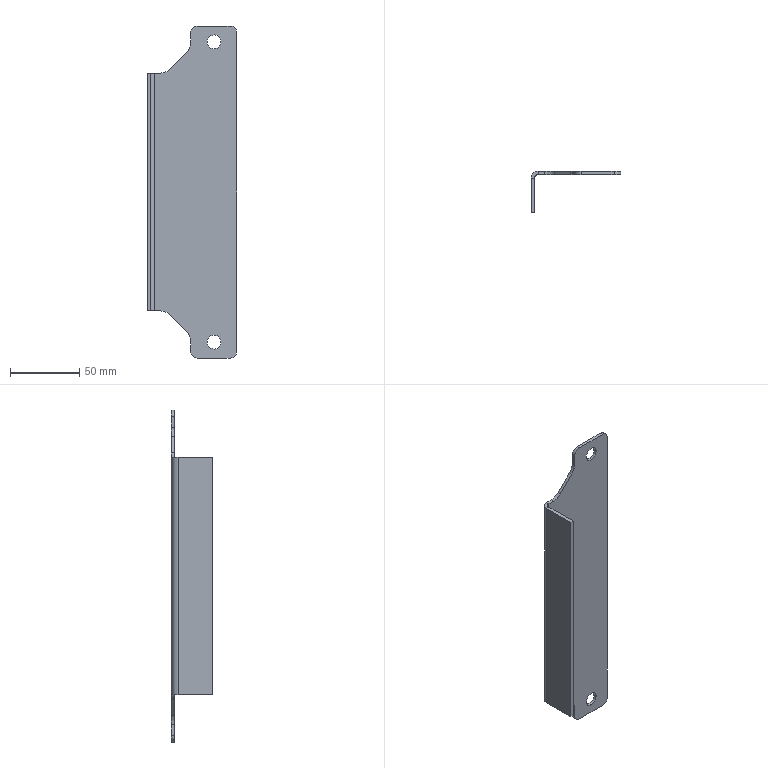Part | SolidWorks | features BaseBody 1, FlatPattern 1, SheetMetal 1, SolidToSheetMetal 1 | 1 solid | 32 faces | box 65 x 30 x 240 mm | volume 41523 mm3 | plane 18 | cylinder 14 | commonest cylinder face diameters 10 x8 20 x4 6 x1 10.6 x1
STEP:
#1=CARTESIAN_POINT('',(1146.2,76.5,704.5));
#2=VERTEX_POINT('',#1);
#3=CARTESIAN_POINT('',(1146.2,76.5,694.5));
#4=VERTEX_POINT('',#3);
#5=CARTESIAN_POINT('',(1146.2,76.5,699.5));
#6=DIRECTION('',(0.,-1.,0.));
#7=DIRECTION('',(0.,0.,-1.));
#8=AXIS2_PLACEMENT_3D('',#5,#6,#7);
#9=CIRCLE('',#8,5.);
#10=EDGE_CURVE('',#2,#4,#9,.T.);
#11=ORIENTED_EDGE('',*,*,#10,.T.);
#12=CARTESIAN_POINT('',(1146.2,78.8,694.5));
#13=VERTEX_POINT('',#12);
#14=CARTESIAN_POINT('',(1146.2,76.5,694.5));
#15=DIRECTION('',(0.,1.,0.));
#16=VECTOR('',#15,1000.);
#17=LINE('',#14,#16);
#18=EDGE_CURVE('',#4,#13,#17,.T.);
#19=ORIENTED_EDGE('',*,*,#18,.T.);
#20=CARTESIAN_POINT('',(1146.2,78.8,704.5));
#21=VERTEX_POINT('',#20);
#22=CARTESIAN_POINT('',(1146.2,78.8,699.5));
#23=DIRECTION('',(0.,-1.,0.));
#24=DIRECTION('',(0.,0.,-1.));
#25=AXIS2_PLACEMENT_3D('',#22,#23,#24);
#26=CIRCLE('',#25,5.);
#27=EDGE_CURVE('',#21,#13,#26,.T.);
#28=ORIENTED_EDGE('',*,*,#27,.F.);
#29=CARTESIAN_POINT('',(1146.2,76.5,704.5));
#30=DIRECTION('',(0.,1.,0.));
#31=VECTOR('',#30,1000.);
#32=LINE('',#29,#31);
#33=EDGE_CURVE('',#2,#21,#32,.T.);
#34=ORIENTED_EDGE('',*,*,#33,.F.);
#35=EDGE_LOOP('',(#11,#19,#28,#34));
#36=FACE_OUTER_BOUND('',#35,.T.);
#37=CARTESIAN_POINT('',(1146.2,76.5,699.5));
#38=DIRECTION('',(0.,1.,0.));
#39=DIRECTION('',(0.,0.,1.));
#40=AXIS2_PLACEMENT_3D('',#37,#38,#39);
#41=CYLINDRICAL_SURFACE('',#40,5.);
#42=ADVANCED_FACE('',(#36),#41,.F.);
#43=CARTESIAN_POINT('',(1146.2,76.5,487.5));
#44=VERTEX_POINT('',#43);
#45=CARTESIAN_POINT('',(1146.2,76.5,477.5));
#46=VERTEX_POINT('',#45);
#47=CARTESIAN_POINT('',(1146.2,76.5,482.5));
#48=DIRECTION('',(0.,-1.,0.));
#49=DIRECTION('',(0.,0.,1.));
#50=AXIS2_PLACEMENT_3D('',#47,#48,#49);
#51=CIRCLE('',#50,5.);
#52=EDGE_CURVE('',#44,#46,#51,.T.);
#53=ORIENTED_EDGE('',*,*,#52,.T.);
#54=CARTESIAN_POINT('',(1146.2,78.8,477.5));
#55=VERTEX_POINT('',#54);
#56=CARTESIAN_POINT('',(1146.2,76.5,477.5));
#57=DIRECTION('',(0.,1.,0.));
#58=VECTOR('',#57,1000.);
#59=LINE('',#56,#58);
#60=EDGE_CURVE('',#46,#55,#59,.T.);
#61=ORIENTED_EDGE('',*,*,#60,.T.);
#62=CARTESIAN_POINT('',(1146.2,78.8,487.5));
#63=VERTEX_POINT('',#62);
#64=CARTESIAN_POINT('',(1146.2,78.8,482.5));
#65=DIRECTION('',(0.,-1.,0.));
#66=DIRECTION('',(0.,0.,1.));
#67=AXIS2_PLACEMENT_3D('',#64,#65,#66);
#68=CIRCLE('',#67,5.);
#69=EDGE_CURVE('',#63,#55,#68,.T.);
#70=ORIENTED_EDGE('',*,*,#69,.F.);
#71=CARTESIAN_POINT('',(1146.2,76.5,487.5));
#72=DIRECTION('',(0.,1.,0.));
#73=VECTOR('',#72,1000.);
#74=LINE('',#71,#73);
#75=EDGE_CURVE('',#44,#63,#74,.T.);
#76=ORIENTED_EDGE('',*,*,#75,.F.);
#77=EDGE_LOOP('',(#53,#61,#70,#76));
#78=FACE_OUTER_BOUND('',#77,.T.);
#79=CARTESIAN_POINT('',(1146.2,76.5,482.5));
#80=DIRECTION('',(0.,1.,0.));
#81=DIRECTION('',(0.,0.,1.));
#82=AXIS2_PLACEMENT_3D('',#79,#80,#81);
#83=CYLINDRICAL_SURFACE('',#82,5.);
#84=ADVANCED_FACE('',(#78),#83,.F.);
#85=CARTESIAN_POINT('',(1107.528,78.8,505.));
#86=VERTEX_POINT('',#85);
#87=CARTESIAN_POINT('',(1107.528,76.5,505.));
#88=VERTEX_POINT('',#87);
#89=CARTESIAN_POINT('',(1107.528,76.5,505.));
#90=DIRECTION('',(0.,-1.,0.));
#91=VECTOR('',#90,1000.);
#92=LINE('',#89,#91);
#93=EDGE_CURVE('',#86,#88,#92,.T.);
#94=ORIENTED_EDGE('',*,*,#93,.F.);
#95=CARTESIAN_POINT('',(1114.599,78.8,502.071));
#96=VERTEX_POINT('',#95);
#97=CARTESIAN_POINT('',(1107.528,78.8,495.));
#98=DIRECTION('',(0.,-1.,0.));
#99=DIRECTION('',(0.,0.,-1.));
#100=AXIS2_PLACEMENT_3D('',#97,#98,#99);
#101=CIRCLE('',#100,10.);
#102=EDGE_CURVE('',#96,#86,#101,.T.);
#103=ORIENTED_EDGE('',*,*,#102,.F.);
#104=CARTESIAN_POINT('',(1114.599,76.5,502.071));
#105=VERTEX_POINT('',#104);
#106=CARTESIAN_POINT('',(1114.599,76.5,502.071));
#107=DIRECTION('',(0.,-1.,0.));
#108=VECTOR('',#107,1000.);
#109=LINE('',#106,#108);
#110=EDGE_CURVE('',#96,#105,#109,.T.);
#111=ORIENTED_EDGE('',*,*,#110,.T.);
#112=CARTESIAN_POINT('',(1107.528,76.5,495.));
#113=DIRECTION('',(0.,-1.,0.));
#114=DIRECTION('',(0.,0.,-1.));
#115=AXIS2_PLACEMENT_3D('',#112,#113,#114);
#116=CIRCLE('',#115,10.);
#117=EDGE_CURVE('',#105,#88,#116,.T.);
#118=ORIENTED_EDGE('',*,*,#117,.T.);
#119=EDGE_LOOP('',(#94,#103,#111,#118));
#120=FACE_OUTER_BOUND('',#119,.T.);
#121=CARTESIAN_POINT('',(1107.528,76.5,495.));
#122=DIRECTION('',(0.,1.,0.));
#123=DIRECTION('',(0.,0.,1.));
#124=AXIS2_PLACEMENT_3D('',#121,#122,#123);
#125=CYLINDRICAL_SURFACE('',#124,10.);
#126=ADVANCED_FACE('',(#120),#125,.F.);
#127=ORIENTED_EDGE('',*,*,#110,.F.);
#128=CARTESIAN_POINT('',(1126.271,78.8,490.399));
#129=VERTEX_POINT('',#128);
#130=CARTESIAN_POINT('',(1126.271,78.8,490.399));
#131=DIRECTION('',(-0.7071,0.,0.7071));
#132=VECTOR('',#131,1000.);
#133=LINE('',#130,#132);
#134=EDGE_CURVE('',#129,#96,#133,.T.);
#135=ORIENTED_EDGE('',*,*,#134,.F.);
#136=CARTESIAN_POINT('',(1126.271,76.5,490.399));
#137=VERTEX_POINT('',#136);
#138=CARTESIAN_POINT('',(1126.271,76.5,490.399));
#139=DIRECTION('',(0.,-1.,0.));
#140=VECTOR('',#139,1000.);
#141=LINE('',#138,#140);
#142=EDGE_CURVE('',#129,#137,#141,.T.);
#143=ORIENTED_EDGE('',*,*,#142,.T.);
#144=CARTESIAN_POINT('',(1126.271,76.5,490.399));
#145=DIRECTION('',(-0.7071,0.,0.7071));
#146=VECTOR('',#145,1000.);
#147=LINE('',#144,#146);
#148=EDGE_CURVE('',#137,#105,#147,.T.);
#149=ORIENTED_EDGE('',*,*,#148,.T.);
#150=EDGE_LOOP('',(#127,#135,#143,#149));
#151=FACE_OUTER_BOUND('',#150,.T.);
#152=CARTESIAN_POINT('',(1126.271,76.5,490.399));
#153=DIRECTION('',(-0.7071,0.,-0.7071));
#154=DIRECTION('',(-0.7071,0.,0.7071));
#155=AXIS2_PLACEMENT_3D('',#152,#153,#154);
#156=PLANE('',#155);
#157=ADVANCED_FACE('',(#151),#156,.T.);
#158=ORIENTED_EDGE('',*,*,#142,.F.);
#159=CARTESIAN_POINT('',(1129.2,78.8,483.328));
#160=VERTEX_POINT('',#159);
#161=CARTESIAN_POINT('',(1119.2,78.8,483.328));
#162=DIRECTION('',(0.,-1.,0.));
#163=DIRECTION('',(1.,0.,0.));
#164=AXIS2_PLACEMENT_3D('',#161,#162,#163);
#165=CIRCLE('',#164,10.);
#166=EDGE_CURVE('',#160,#129,#165,.T.);
#167=ORIENTED_EDGE('',*,*,#166,.F.);
#168=CARTESIAN_POINT('',(1129.2,76.5,483.328));
#169=VERTEX_POINT('',#168);
#170=CARTESIAN_POINT('',(1129.2,76.5,483.328));
#171=DIRECTION('',(0.,-1.,0.));
#172=VECTOR('',#171,1000.);
#173=LINE('',#170,#172);
#174=EDGE_CURVE('',#160,#169,#173,.T.);
#175=ORIENTED_EDGE('',*,*,#174,.T.);
#176=CARTESIAN_POINT('',(1119.2,76.5,483.328));
#177=DIRECTION('',(0.,-1.,0.));
#178=DIRECTION('',(1.,0.,0.));
#179=AXIS2_PLACEMENT_3D('',#176,#177,#178);
#180=CIRCLE('',#179,10.);
#181=EDGE_CURVE('',#169,#137,#180,.T.);
#182=ORIENTED_EDGE('',*,*,#181,.T.);
#183=EDGE_LOOP('',(#158,#167,#175,#182));
#184=FACE_OUTER_BOUND('',#183,.T.);
#185=CARTESIAN_POINT('',(1119.2,76.5,483.328));
#186=DIRECTION('',(0.,1.,0.));
#187=DIRECTION('',(0.,0.,1.));
#188=AXIS2_PLACEMENT_3D('',#185,#186,#187);
#189=CYLINDRICAL_SURFACE('',#188,10.);
#190=ADVANCED_FACE('',(#184),#189,.F.);
#191=ORIENTED_EDGE('',*,*,#174,.F.);
#192=CARTESIAN_POINT('',(1129.2,78.8,476.));
#193=VERTEX_POINT('',#192);
#194=CARTESIAN_POINT('',(1129.2,78.8,711.));
#195=DIRECTION('',(0.,0.,1.));
#196=VECTOR('',#195,1000.);
#197=LINE('',#194,#196);
#198=EDGE_CURVE('',#193,#160,#197,.T.);
#199=ORIENTED_EDGE('',*,*,#198,.F.);
#200=CARTESIAN_POINT('',(1129.2,76.5,476.));
#201=VERTEX_POINT('',#200);
#202=CARTESIAN_POINT('',(1129.2,76.5,476.));
#203=DIRECTION('',(0.,-1.,0.));
#204=VECTOR('',#203,1000.);
#205=LINE('',#202,#204);
#206=EDGE_CURVE('',#193,#201,#205,.T.);
#207=ORIENTED_EDGE('',*,*,#206,.T.);
#208=CARTESIAN_POINT('',(1129.2,76.5,591.));
#209=DIRECTION('',(0.,0.,1.));
#210=VECTOR('',#209,1000.);
#211=LINE('',#208,#210);
#212=EDGE_CURVE('',#201,#169,#211,.T.);
#213=ORIENTED_EDGE('',*,*,#212,.T.);
#214=EDGE_LOOP('',(#191,#199,#207,#213));
#215=FACE_OUTER_BOUND('',#214,.T.);
#216=CARTESIAN_POINT('',(1129.2,76.5,591.));
#217=DIRECTION('',(-1.,0.,0.));
#218=DIRECTION('',(0.,0.,1.));
#219=AXIS2_PLACEMENT_3D('',#216,#217,#218);
#220=PLANE('',#219);
#221=ADVANCED_FACE('',(#215),#220,.T.);
#222=ORIENTED_EDGE('',*,*,#206,.F.);
#223=CARTESIAN_POINT('',(1134.2,78.8,471.));
#224=VERTEX_POINT('',#223);
#225=CARTESIAN_POINT('',(1134.2,78.8,476.));
#226=DIRECTION('',(0.,1.,0.));
#227=DIRECTION('',(0.,0.,1.));
#228=AXIS2_PLACEMENT_3D('',#225,#226,#227);
#229=CIRCLE('',#228,5.);
#230=EDGE_CURVE('',#224,#193,#229,.T.);
#231=ORIENTED_EDGE('',*,*,#230,.F.);
#232=CARTESIAN_POINT('',(1134.2,76.5,471.));
#233=VERTEX_POINT('',#232);
#234=CARTESIAN_POINT('',(1134.2,76.5,471.));
#235=DIRECTION('',(0.,-1.,0.));
#236=VECTOR('',#235,1000.);
#237=LINE('',#234,#236);
#238=EDGE_CURVE('',#224,#233,#237,.T.);
#239=ORIENTED_EDGE('',*,*,#238,.T.);
#240=CARTESIAN_POINT('',(1134.2,76.5,476.));
#241=DIRECTION('',(0.,1.,0.));
#242=DIRECTION('',(0.,0.,1.));
#243=AXIS2_PLACEMENT_3D('',#240,#241,#242);
#244=CIRCLE('',#243,5.);
#245=EDGE_CURVE('',#233,#201,#244,.T.);
#246=ORIENTED_EDGE('',*,*,#245,.T.);
#247=EDGE_LOOP('',(#222,#231,#239,#246));
#248=FACE_OUTER_BOUND('',#247,.T.);
#249=CARTESIAN_POINT('',(1134.2,76.5,476.));
#250=DIRECTION('',(0.,1.,0.));
#251=DIRECTION('',(0.,0.,1.));
#252=AXIS2_PLACEMENT_3D('',#249,#250,#251);
#253=CYLINDRICAL_SURFACE('',#252,5.);
#254=ADVANCED_FACE('',(#248),#253,.T.);
#255=ORIENTED_EDGE('',*,*,#238,.F.);
#256=CARTESIAN_POINT('',(1157.7,78.8,471.));
#257=VERTEX_POINT('',#256);
#258=CARTESIAN_POINT('',(1103.,78.8,471.));
#259=DIRECTION('',(-1.,0.,0.));
#260=VECTOR('',#259,1000.);
#261=LINE('',#258,#260);
#262=EDGE_CURVE('',#257,#224,#261,.T.);
#263=ORIENTED_EDGE('',*,*,#262,.F.);
#264=CARTESIAN_POINT('',(1157.7,76.5,471.));
#265=VERTEX_POINT('',#264);
#266=CARTESIAN_POINT('',(1157.7,76.5,471.));
#267=DIRECTION('',(0.,-1.,0.));
#268=VECTOR('',#267,1000.);
#269=LINE('',#266,#268);
#270=EDGE_CURVE('',#257,#265,#269,.T.);
#271=ORIENTED_EDGE('',*,*,#270,.T.);
#272=CARTESIAN_POINT('',(1132.85,76.5,471.));
#273=DIRECTION('',(-1.,0.,0.));
#274=VECTOR('',#273,1000.);
#275=LINE('',#272,#274);
#276=EDGE_CURVE('',#265,#233,#275,.T.);
#277=ORIENTED_EDGE('',*,*,#276,.T.);
#278=EDGE_LOOP('',(#255,#263,#271,#277));
#279=FACE_OUTER_BOUND('',#278,.T.);
#280=CARTESIAN_POINT('',(1132.85,76.5,471.));
#281=DIRECTION('',(0.,0.,-1.));
#282=DIRECTION('',(-1.,0.,0.));
#283=AXIS2_PLACEMENT_3D('',#280,#281,#282);
#284=PLANE('',#283);
#285=ADVANCED_FACE('',(#279),#284,.T.);
#286=ORIENTED_EDGE('',*,*,#270,.F.);
#287=CARTESIAN_POINT('',(1162.7,78.8,476.));
#288=VERTEX_POINT('',#287);
#289=CARTESIAN_POINT('',(1157.7,78.8,476.));
#290=DIRECTION('',(0.,1.,0.));
#291=DIRECTION('',(0.,0.,1.));
#292=AXIS2_PLACEMENT_3D('',#289,#290,#291);
#293=CIRCLE('',#292,5.);
#294=EDGE_CURVE('',#288,#257,#293,.T.);
#295=ORIENTED_EDGE('',*,*,#294,.F.);
#296=CARTESIAN_POINT('',(1162.7,76.5,476.));
#297=VERTEX_POINT('',#296);
#298=CARTESIAN_POINT('',(1162.7,76.5,476.));
#299=DIRECTION('',(0.,-1.,0.));
#300=VECTOR('',#299,1000.);
#301=LINE('',#298,#300);
#302=EDGE_CURVE('',#288,#297,#301,.T.);
#303=ORIENTED_EDGE('',*,*,#302,.T.);
#304=CARTESIAN_POINT('',(1157.7,76.5,476.));
#305=DIRECTION('',(0.,1.,0.));
#306=DIRECTION('',(0.,0.,1.));
#307=AXIS2_PLACEMENT_3D('',#304,#305,#306);
#308=CIRCLE('',#307,5.);
#309=EDGE_CURVE('',#297,#265,#308,.T.);
#310=ORIENTED_EDGE('',*,*,#309,.T.);
#311=EDGE_LOOP('',(#286,#295,#303,#310));
#312=FACE_OUTER_BOUND('',#311,.T.);
#313=CARTESIAN_POINT('',(1157.7,76.5,476.));
#314=DIRECTION('',(0.,1.,0.));
#315=DIRECTION('',(0.,0.,1.));
#316=AXIS2_PLACEMENT_3D('',#313,#314,#315);
#317=CYLINDRICAL_SURFACE('',#316,5.);
#318=ADVANCED_FACE('',(#312),#317,.T.);
#319=ORIENTED_EDGE('',*,*,#302,.F.);
#320=CARTESIAN_POINT('',(1162.7,78.8,706.));
#321=VERTEX_POINT('',#320);
#322=CARTESIAN_POINT('',(1162.7,78.8,711.));
#323=DIRECTION('',(0.,0.,-1.));
#324=VECTOR('',#323,1000.);
#325=LINE('',#322,#324);
#326=EDGE_CURVE('',#321,#288,#325,.T.);
#327=ORIENTED_EDGE('',*,*,#326,.F.);
#328=CARTESIAN_POINT('',(1162.7,76.5,706.));
#329=VERTEX_POINT('',#328);
#330=CARTESIAN_POINT('',(1162.7,76.5,706.));
#331=DIRECTION('',(0.,-1.,0.));
#332=VECTOR('',#331,1000.);
#333=LINE('',#330,#332);
#334=EDGE_CURVE('',#321,#329,#333,.T.);
#335=ORIENTED_EDGE('',*,*,#334,.T.);
#336=CARTESIAN_POINT('',(1162.7,76.5,591.));
#337=DIRECTION('',(0.,0.,-1.));
#338=VECTOR('',#337,1000.);
#339=LINE('',#336,#338);
#340=EDGE_CURVE('',#329,#297,#339,.T.);
#341=ORIENTED_EDGE('',*,*,#340,.T.);
#342=EDGE_LOOP('',(#319,#327,#335,#341));
#343=FACE_OUTER_BOUND('',#342,.T.);
#344=CARTESIAN_POINT('',(1162.7,76.5,591.));
#345=DIRECTION('',(1.,0.,0.));
#346=DIRECTION('',(0.,0.,-1.));
#347=AXIS2_PLACEMENT_3D('',#344,#345,#346);
#348=PLANE('',#347);
#349=ADVANCED_FACE('',(#343),#348,.T.);
#350=ORIENTED_EDGE('',*,*,#334,.F.);
#351=CARTESIAN_POINT('',(1157.7,78.8,711.));
#352=VERTEX_POINT('',#351);
#353=CARTESIAN_POINT('',(1157.7,78.8,706.));
#354=DIRECTION('',(0.,1.,0.));
#355=DIRECTION('',(0.,0.,1.));
#356=AXIS2_PLACEMENT_3D('',#353,#354,#355);
#357=CIRCLE('',#356,5.);
#358=EDGE_CURVE('',#352,#321,#357,.T.);
#359=ORIENTED_EDGE('',*,*,#358,.F.);
#360=CARTESIAN_POINT('',(1157.7,76.5,711.));
#361=VERTEX_POINT('',#360);
#362=CARTESIAN_POINT('',(1157.7,76.5,711.));
#363=DIRECTION('',(0.,-1.,0.));
#364=VECTOR('',#363,1000.);
#365=LINE('',#362,#364);
#366=EDGE_CURVE('',#352,#361,#365,.T.);
#367=ORIENTED_EDGE('',*,*,#366,.T.);
#368=CARTESIAN_POINT('',(1157.7,76.5,706.));
#369=DIRECTION('',(0.,1.,0.));
#370=DIRECTION('',(0.,0.,1.));
#371=AXIS2_PLACEMENT_3D('',#368,#369,#370);
#372=CIRCLE('',#371,5.);
#373=EDGE_CURVE('',#361,#329,#372,.T.);
#374=ORIENTED_EDGE('',*,*,#373,.T.);
#375=EDGE_LOOP('',(#350,#359,#367,#374));
#376=FACE_OUTER_BOUND('',#375,.T.);
#377=CARTESIAN_POINT('',(1157.7,76.5,706.));
#378=DIRECTION('',(0.,1.,0.));
#379=DIRECTION('',(0.,0.,1.));
#380=AXIS2_PLACEMENT_3D('',#377,#378,#379);
#381=CYLINDRICAL_SURFACE('',#380,5.);
#382=ADVANCED_FACE('',(#376),#381,.T.);
#383=ORIENTED_EDGE('',*,*,#366,.F.);
#384=CARTESIAN_POINT('',(1134.2,78.8,711.));
#385=VERTEX_POINT('',#384);
#386=CARTESIAN_POINT('',(1103.,78.8,711.));
#387=DIRECTION('',(1.,0.,0.));
#388=VECTOR('',#387,1000.);
#389=LINE('',#386,#388);
#390=EDGE_CURVE('',#385,#352,#389,.T.);
#391=ORIENTED_EDGE('',*,*,#390,.F.);
#392=CARTESIAN_POINT('',(1134.2,76.5,711.));
#393=VERTEX_POINT('',#392);
#394=CARTESIAN_POINT('',(1134.2,76.5,711.));
#395=DIRECTION('',(0.,-1.,0.));
#396=VECTOR('',#395,1000.);
#397=LINE('',#394,#396);
#398=EDGE_CURVE('',#385,#393,#397,.T.);
#399=ORIENTED_EDGE('',*,*,#398,.T.);
#400=CARTESIAN_POINT('',(1132.85,76.5,711.));
#401=DIRECTION('',(1.,0.,0.));
#402=VECTOR('',#401,1000.);
#403=LINE('',#400,#402);
#404=EDGE_CURVE('',#393,#361,#403,.T.);
#405=ORIENTED_EDGE('',*,*,#404,.T.);
#406=EDGE_LOOP('',(#383,#391,#399,#405));
#407=FACE_OUTER_BOUND('',#406,.T.);
#408=CARTESIAN_POINT('',(1132.85,76.5,711.));
#409=DIRECTION('',(0.,0.,1.));
#410=DIRECTION('',(1.,0.,0.));
#411=AXIS2_PLACEMENT_3D('',#408,#409,#410);
#412=PLANE('',#411);
#413=ADVANCED_FACE('',(#407),#412,.T.);
#414=ORIENTED_EDGE('',*,*,#398,.F.);
#415=CARTESIAN_POINT('',(1129.2,78.8,706.));
#416=VERTEX_POINT('',#415);
#417=CARTESIAN_POINT('',(1134.2,78.8,706.));
#418=DIRECTION('',(0.,1.,0.));
#419=DIRECTION('',(0.,0.,1.));
#420=AXIS2_PLACEMENT_3D('',#417,#418,#419);
#421=CIRCLE('',#420,5.);
#422=EDGE_CURVE('',#416,#385,#421,.T.);
#423=ORIENTED_EDGE('',*,*,#422,.F.);
#424=CARTESIAN_POINT('',(1129.2,76.5,706.));
#425=VERTEX_POINT('',#424);
#426=CARTESIAN_POINT('',(1129.2,76.5,706.));
#427=DIRECTION('',(0.,-1.,0.));
#428=VECTOR('',#427,1000.);
#429=LINE('',#426,#428);
#430=EDGE_CURVE('',#416,#425,#429,.T.);
#431=ORIENTED_EDGE('',*,*,#430,.T.);
#432=CARTESIAN_POINT('',(1134.2,76.5,706.));
#433=DIRECTION('',(0.,1.,0.));
#434=DIRECTION('',(0.,0.,1.));
#435=AXIS2_PLACEMENT_3D('',#432,#433,#434);
#436=CIRCLE('',#435,5.);
#437=EDGE_CURVE('',#425,#393,#436,.T.);
#438=ORIENTED_EDGE('',*,*,#437,.T.);
#439=EDGE_LOOP('',(#414,#423,#431,#438));
#440=FACE_OUTER_BOUND('',#439,.T.);
#441=CARTESIAN_POINT('',(1134.2,76.5,706.));
#442=DIRECTION('',(0.,1.,0.));
#443=DIRECTION('',(0.,0.,1.));
#444=AXIS2_PLACEMENT_3D('',#441,#442,#443);
#445=CYLINDRICAL_SURFACE('',#444,5.);
#446=ADVANCED_FACE('',(#440),#445,.T.);
#447=ORIENTED_EDGE('',*,*,#430,.F.);
#448=CARTESIAN_POINT('',(1129.2,78.8,698.672));
#449=VERTEX_POINT('',#448);
#450=CARTESIAN_POINT('',(1129.2,78.8,711.));
#451=DIRECTION('',(0.,0.,1.));
#452=VECTOR('',#451,1000.);
#453=LINE('',#450,#452);
#454=EDGE_CURVE('',#449,#416,#453,.T.);
#455=ORIENTED_EDGE('',*,*,#454,.F.);
#456=CARTESIAN_POINT('',(1129.2,76.5,698.672));
#457=VERTEX_POINT('',#456);
#458=CARTESIAN_POINT('',(1129.2,76.5,698.672));
#459=DIRECTION('',(0.,-1.,0.));
#460=VECTOR('',#459,1000.);
#461=LINE('',#458,#460);
#462=EDGE_CURVE('',#449,#457,#461,.T.);
#463=ORIENTED_EDGE('',*,*,#462,.T.);
#464=CARTESIAN_POINT('',(1129.2,76.5,591.));
#465=DIRECTION('',(0.,0.,1.));
#466=VECTOR('',#465,1000.);
#467=LINE('',#464,#466);
#468=EDGE_CURVE('',#457,#425,#467,.T.);
#469=ORIENTED_EDGE('',*,*,#468,.T.);
#470=EDGE_LOOP('',(#447,#455,#463,#469));
#471=FACE_OUTER_BOUND('',#470,.T.);
#472=CARTESIAN_POINT('',(1129.2,76.5,591.));
#473=DIRECTION('',(-1.,0.,0.));
#474=DIRECTION('',(0.,0.,1.));
#475=AXIS2_PLACEMENT_3D('',#472,#473,#474);
#476=PLANE('',#475);
#477=ADVANCED_FACE('',(#471),#476,.T.);
#478=ORIENTED_EDGE('',*,*,#462,.F.);
#479=CARTESIAN_POINT('',(1126.271,78.8,691.601));
#480=VERTEX_POINT('',#479);
#481=CARTESIAN_POINT('',(1119.2,78.8,698.672));
#482=DIRECTION('',(0.,-1.,0.));
#483=DIRECTION('',(-1.,0.,0.));
#484=AXIS2_PLACEMENT_3D('',#481,#482,#483);
#485=CIRCLE('',#484,10.);
#486=EDGE_CURVE('',#480,#449,#485,.T.);
#487=ORIENTED_EDGE('',*,*,#486,.F.);
#488=CARTESIAN_POINT('',(1126.271,76.5,691.601));
#489=VERTEX_POINT('',#488);
#490=CARTESIAN_POINT('',(1126.271,76.5,691.601));
#491=DIRECTION('',(0.,-1.,0.));
#492=VECTOR('',#491,1000.);
#493=LINE('',#490,#492);
#494=EDGE_CURVE('',#480,#489,#493,.T.);
#495=ORIENTED_EDGE('',*,*,#494,.T.);
#496=CARTESIAN_POINT('',(1119.2,76.5,698.672));
#497=DIRECTION('',(0.,-1.,0.));
#498=DIRECTION('',(-1.,0.,0.));
#499=AXIS2_PLACEMENT_3D('',#496,#497,#498);
#500=CIRCLE('',#499,10.);
#501=EDGE_CURVE('',#489,#457,#500,.T.);
#502=ORIENTED_EDGE('',*,*,#501,.T.);
#503=EDGE_LOOP('',(#478,#487,#495,#502));
#504=FACE_OUTER_BOUND('',#503,.T.);
#505=CARTESIAN_POINT('',(1119.2,76.5,698.672));
#506=DIRECTION('',(0.,1.,0.));
#507=DIRECTION('',(0.,0.,1.));
#508=AXIS2_PLACEMENT_3D('',#505,#506,#507);
#509=CYLINDRICAL_SURFACE('',#508,10.);
#510=ADVANCED_FACE('',(#504),#509,.F.);
#511=ORIENTED_EDGE('',*,*,#494,.F.);
#512=CARTESIAN_POINT('',(1114.599,78.8,679.929));
#513=VERTEX_POINT('',#512);
#514=CARTESIAN_POINT('',(1126.271,78.8,691.601));
#515=DIRECTION('',(0.7071,0.,0.7071));
#516=VECTOR('',#515,1000.);
#517=LINE('',#514,#516);
#518=EDGE_CURVE('',#513,#480,#517,.T.);
#519=ORIENTED_EDGE('',*,*,#518,.F.);
#520=CARTESIAN_POINT('',(1114.599,76.5,679.929));
#521=VERTEX_POINT('',#520);
#522=CARTESIAN_POINT('',(1114.599,76.5,679.929));
#523=DIRECTION('',(0.,-1.,0.));
#524=VECTOR('',#523,1000.);
#525=LINE('',#522,#524);
#526=EDGE_CURVE('',#513,#521,#525,.T.);
#527=ORIENTED_EDGE('',*,*,#526,.T.);
#528=CARTESIAN_POINT('',(1126.271,76.5,691.601));
#529=DIRECTION('',(0.7071,0.,0.7071));
#530=VECTOR('',#529,1000.);
#531=LINE('',#528,#530);
#532=EDGE_CURVE('',#521,#489,#531,.T.);
#533=ORIENTED_EDGE('',*,*,#532,.T.);
#534=EDGE_LOOP('',(#511,#519,#527,#533));
#535=FACE_OUTER_BOUND('',#534,.T.);
#536=CARTESIAN_POINT('',(1126.271,76.5,691.601));
#537=DIRECTION('',(0.7071,0.,-0.7071));
#538=DIRECTION('',(-0.7071,0.,-0.7071));
#539=AXIS2_PLACEMENT_3D('',#536,#537,#538);
#540=PLANE('',#539);
#541=ADVANCED_FACE('',(#535),#540,.F.);
#542=ORIENTED_EDGE('',*,*,#526,.F.);
#543=CARTESIAN_POINT('',(1107.528,78.8,677.));
#544=VERTEX_POINT('',#543);
#545=CARTESIAN_POINT('',(1107.528,78.8,687.));
#546=DIRECTION('',(0.,-1.,0.));
#547=DIRECTION('',(0.,0.,1.));
#548=AXIS2_PLACEMENT_3D('',#545,#546,#547);
#549=CIRCLE('',#548,10.);
#550=EDGE_CURVE('',#544,#513,#549,.T.);
#551=ORIENTED_EDGE('',*,*,#550,.F.);
#552=CARTESIAN_POINT('',(1107.528,76.5,677.));
#553=VERTEX_POINT('',#552);
#554=CARTESIAN_POINT('',(1107.528,76.5,677.));
#555=DIRECTION('',(0.,-1.,0.));
#556=VECTOR('',#555,1000.);
#557=LINE('',#554,#556);
#558=EDGE_CURVE('',#544,#553,#557,.T.);
#559=ORIENTED_EDGE('',*,*,#558,.T.);
#560=CARTESIAN_POINT('',(1107.528,76.5,687.));
#561=DIRECTION('',(0.,-1.,0.));
#562=DIRECTION('',(0.,0.,1.));
#563=AXIS2_PLACEMENT_3D('',#560,#561,#562);
#564=CIRCLE('',#563,10.);
#565=EDGE_CURVE('',#553,#521,#564,.T.);
#566=ORIENTED_EDGE('',*,*,#565,.T.);
#567=EDGE_LOOP('',(#542,#551,#559,#566));
#568=FACE_OUTER_BOUND('',#567,.T.);
#569=CARTESIAN_POINT('',(1107.528,76.5,687.));
#570=DIRECTION('',(0.,1.,0.));
#571=DIRECTION('',(0.,0.,1.));
#572=AXIS2_PLACEMENT_3D('',#569,#570,#571);
#573=CYLINDRICAL_SURFACE('',#572,10.);
#574=ADVANCED_FACE('',(#568),#573,.F.);
#575=ORIENTED_EDGE('',*,*,#558,.F.);
#576=CARTESIAN_POINT('',(1103.,78.8,677.));
#577=VERTEX_POINT('',#576);
#578=CARTESIAN_POINT('',(1103.,78.8,677.));
#579=DIRECTION('',(1.,0.,0.));
#580=VECTOR('',#579,1000.);
#581=LINE('',#578,#580);
#582=EDGE_CURVE('',#577,#544,#581,.T.);
#583=ORIENTED_EDGE('',*,*,#582,.F.);
#584=CARTESIAN_POINT('',(1103.,76.5,677.));
#585=VERTEX_POINT('',#584);
#586=CARTESIAN_POINT('',(1103.,76.5,677.));
#587=DIRECTION('',(0.,-1.,0.));
#588=VECTOR('',#587,1000.);
#589=LINE('',#586,#588);
#590=EDGE_CURVE('',#577,#585,#589,.T.);
#591=ORIENTED_EDGE('',*,*,#590,.T.);
#592=CARTESIAN_POINT('',(1132.85,76.5,677.));
#593=DIRECTION('',(1.,0.,0.));
#594=VECTOR('',#593,1000.);
#595=LINE('',#592,#594);
#596=EDGE_CURVE('',#585,#553,#595,.T.);
#597=ORIENTED_EDGE('',*,*,#596,.T.);
#598=EDGE_LOOP('',(#575,#583,#591,#597));
#599=FACE_OUTER_BOUND('',#598,.T.);
#600=CARTESIAN_POINT('',(1132.85,76.5,677.));
#601=DIRECTION('',(0.,0.,1.));
#602=DIRECTION('',(1.,0.,0.));
#603=AXIS2_PLACEMENT_3D('',#600,#601,#602);
#604=PLANE('',#603);
#605=ADVANCED_FACE('',(#599),#604,.T.);
#606=ORIENTED_EDGE('',*,*,#590,.F.);
#607=CARTESIAN_POINT('',(1097.7,73.5,677.));
#608=VERTEX_POINT('',#607);
#609=CARTESIAN_POINT('',(1103.,73.5,677.));
#610=DIRECTION('',(0.,0.,1.));
#611=DIRECTION('',(-1.,0.,0.));
#612=AXIS2_PLACEMENT_3D('',#609,#610,#611);
#613=CIRCLE('',#612,5.3);
#614=EDGE_CURVE('',#577,#608,#613,.T.);
#615=ORIENTED_EDGE('',*,*,#614,.T.);
#616=CARTESIAN_POINT('',(1100.,73.5,677.));
#617=VERTEX_POINT('',#616);
#618=CARTESIAN_POINT('',(1100.,73.5,677.));
#619=DIRECTION('',(1.,0.,0.));
#620=VECTOR('',#619,1000.);
#621=LINE('',#618,#620);
#622=EDGE_CURVE('',#608,#617,#621,.T.);
#623=ORIENTED_EDGE('',*,*,#622,.T.);
#624=CARTESIAN_POINT('',(1103.,73.5,677.));
#625=DIRECTION('',(0.,0.,1.));
#626=DIRECTION('',(-1.,0.,0.));
#627=AXIS2_PLACEMENT_3D('',#624,#625,#626);
#628=CIRCLE('',#627,3.);
#629=EDGE_CURVE('',#585,#617,#628,.T.);
#630=ORIENTED_EDGE('',*,*,#629,.F.);
#631=EDGE_LOOP('',(#606,#615,#623,#630));
#632=FACE_OUTER_BOUND('',#631,.T.);
#633=CARTESIAN_POINT('',(1103.,73.5,677.));
#634=DIRECTION('',(0.,0.,1.));
#635=DIRECTION('',(1.,0.,0.));
#636=AXIS2_PLACEMENT_3D('',#633,#634,#635);
#637=PLANE('',#636);
#638=ADVANCED_FACE('',(#632),#637,.T.);
#639=ORIENTED_EDGE('',*,*,#622,.F.);
#640=CARTESIAN_POINT('',(1097.7,48.8,677.));
#641=VERTEX_POINT('',#640);
#642=CARTESIAN_POINT('',(1097.7,48.8,677.));
#643=DIRECTION('',(0.,1.,0.));
#644=VECTOR('',#643,1000.);
#645=LINE('',#642,#644);
#646=EDGE_CURVE('',#641,#608,#645,.T.);
#647=ORIENTED_EDGE('',*,*,#646,.F.);
#648=CARTESIAN_POINT('',(1100.,48.8,677.));
#649=VERTEX_POINT('',#648);
#650=CARTESIAN_POINT('',(1100.,48.8,677.));
#651=DIRECTION('',(1.,0.,0.));
#652=VECTOR('',#651,1000.);
#653=LINE('',#650,#652);
#654=EDGE_CURVE('',#641,#649,#653,.T.);
#655=ORIENTED_EDGE('',*,*,#654,.T.);
#656=CARTESIAN_POINT('',(1100.,61.15,677.));
#657=DIRECTION('',(0.,1.,0.));
#658=VECTOR('',#657,1000.);
#659=LINE('',#656,#658);
#660=EDGE_CURVE('',#649,#617,#659,.T.);
#661=ORIENTED_EDGE('',*,*,#660,.T.);
#662=EDGE_LOOP('',(#639,#647,#655,#661));
#663=FACE_OUTER_BOUND('',#662,.T.);
#664=CARTESIAN_POINT('',(1100.,61.15,677.));
#665=DIRECTION('',(0.,0.,1.));
#666=DIRECTION('',(0.,1.,0.));
#667=AXIS2_PLACEMENT_3D('',#664,#665,#666);
#668=PLANE('',#667);
#669=ADVANCED_FACE('',(#663),#668,.T.);
#670=ORIENTED_EDGE('',*,*,#654,.F.);
#671=CARTESIAN_POINT('',(1097.7,48.8,505.));
#672=VERTEX_POINT('',#671);
#673=CARTESIAN_POINT('',(1097.7,48.8,505.));
#674=DIRECTION('',(0.,0.,1.));
#675=VECTOR('',#674,1000.);
#676=LINE('',#673,#675);
#677=EDGE_CURVE('',#672,#641,#676,.T.);
#678=ORIENTED_EDGE('',*,*,#677,.F.);
#679=CARTESIAN_POINT('',(1100.,48.8,505.));
#680=VERTEX_POINT('',#679);
#681=CARTESIAN_POINT('',(1100.,48.8,505.));
#682=DIRECTION('',(1.,0.,0.));
#683=VECTOR('',#682,1000.);
#684=LINE('',#681,#683);
#685=EDGE_CURVE('',#672,#680,#684,.T.);
#686=ORIENTED_EDGE('',*,*,#685,.T.);
#687=CARTESIAN_POINT('',(1100.,48.8,591.));
#688=DIRECTION('',(0.,0.,1.));
#689=VECTOR('',#688,1000.);
#690=LINE('',#687,#689);
#691=EDGE_CURVE('',#680,#649,#690,.T.);
#692=ORIENTED_EDGE('',*,*,#691,.T.);
#693=EDGE_LOOP('',(#670,#678,#686,#692));
#694=FACE_OUTER_BOUND('',#693,.T.);
#695=CARTESIAN_POINT('',(1100.,48.8,591.));
#696=DIRECTION('',(0.,-1.,0.));
#697=DIRECTION('',(0.,0.,1.));
#698=AXIS2_PLACEMENT_3D('',#695,#696,#697);
#699=PLANE('',#698);
#700=ADVANCED_FACE('',(#694),#699,.T.);
#701=ORIENTED_EDGE('',*,*,#685,.F.);
#702=CARTESIAN_POINT('',(1097.7,73.5,505.));
#703=VERTEX_POINT('',#702);
#704=CARTESIAN_POINT('',(1097.7,48.8,505.));
#705=DIRECTION('',(0.,-1.,0.));
#706=VECTOR('',#705,1000.);
#707=LINE('',#704,#706);
#708=EDGE_CURVE('',#703,#672,#707,.T.);
#709=ORIENTED_EDGE('',*,*,#708,.F.);
#710=CARTESIAN_POINT('',(1100.,73.5,505.));
#711=VERTEX_POINT('',#710);
#712=CARTESIAN_POINT('',(1100.,73.5,505.));
#713=DIRECTION('',(1.,0.,0.));
#714=VECTOR('',#713,1000.);
#715=LINE('',#712,#714);
#716=EDGE_CURVE('',#703,#711,#715,.T.);
#717=ORIENTED_EDGE('',*,*,#716,.T.);
#718=CARTESIAN_POINT('',(1100.,63.8,505.));
#719=DIRECTION('',(0.,-1.,0.));
#720=VECTOR('',#719,1000.);
#721=LINE('',#718,#720);
#722=EDGE_CURVE('',#711,#680,#721,.T.);
#723=ORIENTED_EDGE('',*,*,#722,.T.);
#724=EDGE_LOOP('',(#701,#709,#717,#723));
#725=FACE_OUTER_BOUND('',#724,.T.);
#726=CARTESIAN_POINT('',(1100.,63.8,505.));
#727=DIRECTION('',(0.,0.,-1.));
#728=DIRECTION('',(0.,-1.,0.));
#729=AXIS2_PLACEMENT_3D('',#726,#727,#728);
#730=PLANE('',#729);
#731=ADVANCED_FACE('',(#725),#730,.T.);
#732=ORIENTED_EDGE('',*,*,#716,.F.);
#733=CARTESIAN_POINT('',(1103.,78.8,505.));
#734=VERTEX_POINT('',#733);
#735=CARTESIAN_POINT('',(1103.,73.5,505.));
#736=DIRECTION('',(0.,0.,1.));
#737=DIRECTION('',(-1.,0.,0.));
#738=AXIS2_PLACEMENT_3D('',#735,#736,#737);
#739=CIRCLE('',#738,5.3);
#740=EDGE_CURVE('',#734,#703,#739,.T.);
#741=ORIENTED_EDGE('',*,*,#740,.F.);
#742=CARTESIAN_POINT('',(1103.,76.5,505.));
#743=VERTEX_POINT('',#742);
#744=CARTESIAN_POINT('',(1103.,76.5,505.));
#745=DIRECTION('',(0.,-1.,0.));
#746=VECTOR('',#745,1000.);
#747=LINE('',#744,#746);
#748=EDGE_CURVE('',#734,#743,#747,.T.);
#749=ORIENTED_EDGE('',*,*,#748,.T.);
#750=CARTESIAN_POINT('',(1103.,73.5,505.));
#751=DIRECTION('',(0.,0.,1.));
#752=DIRECTION('',(-1.,0.,0.));
#753=AXIS2_PLACEMENT_3D('',#750,#751,#752);
#754=CIRCLE('',#753,3.);
#755=EDGE_CURVE('',#743,#711,#754,.T.);
#756=ORIENTED_EDGE('',*,*,#755,.T.);
#757=EDGE_LOOP('',(#732,#741,#749,#756));
#758=FACE_OUTER_BOUND('',#757,.T.);
#759=CARTESIAN_POINT('',(1103.,73.5,505.));
#760=DIRECTION('',(0.,0.,1.));
#761=DIRECTION('',(1.,0.,0.));
#762=AXIS2_PLACEMENT_3D('',#759,#760,#761);
#763=PLANE('',#762);
#764=ADVANCED_FACE('',(#758),#763,.F.);
#765=ORIENTED_EDGE('',*,*,#60,.F.);
#766=CARTESIAN_POINT('',(1146.2,76.5,482.5));
#767=DIRECTION('',(0.,-1.,0.));
#768=DIRECTION('',(0.,0.,1.));
#769=AXIS2_PLACEMENT_3D('',#766,#767,#768);
#770=CIRCLE('',#769,5.);
#771=EDGE_CURVE('',#46,#44,#770,.T.);
#772=ORIENTED_EDGE('',*,*,#771,.T.);
#773=ORIENTED_EDGE('',*,*,#75,.T.);
#774=CARTESIAN_POINT('',(1146.2,78.8,482.5));
#775=DIRECTION('',(0.,-1.,0.));
#776=DIRECTION('',(0.,0.,1.));
#777=AXIS2_PLACEMENT_3D('',#774,#775,#776);
#778=CIRCLE('',#777,5.);
#779=EDGE_CURVE('',#55,#63,#778,.T.);
#780=ORIENTED_EDGE('',*,*,#779,.F.);
#781=EDGE_LOOP('',(#765,#772,#773,#780));
#782=FACE_OUTER_BOUND('',#781,.T.);
#783=CARTESIAN_POINT('',(1146.2,76.5,482.5));
#784=DIRECTION('',(0.,1.,0.));
#785=DIRECTION('',(0.,0.,1.));
#786=AXIS2_PLACEMENT_3D('',#783,#784,#785);
#787=CYLINDRICAL_SURFACE('',#786,5.);
#788=ADVANCED_FACE('',(#782),#787,.F.);
#789=ORIENTED_EDGE('',*,*,#18,.F.);
#790=CARTESIAN_POINT('',(1146.2,76.5,699.5));
#791=DIRECTION('',(0.,-1.,0.));
#792=DIRECTION('',(0.,0.,-1.));
#793=AXIS2_PLACEMENT_3D('',#790,#791,#792);
#794=CIRCLE('',#793,5.);
#795=EDGE_CURVE('',#4,#2,#794,.T.);
#796=ORIENTED_EDGE('',*,*,#795,.T.);
#797=ORIENTED_EDGE('',*,*,#33,.T.);
#798=CARTESIAN_POINT('',(1146.2,78.8,699.5));
#799=DIRECTION('',(0.,-1.,0.));
#800=DIRECTION('',(0.,0.,-1.));
#801=AXIS2_PLACEMENT_3D('',#798,#799,#800);
#802=CIRCLE('',#801,5.);
#803=EDGE_CURVE('',#13,#21,#802,.T.);
#804=ORIENTED_EDGE('',*,*,#803,.F.);
#805=EDGE_LOOP('',(#789,#796,#797,#804));
#806=FACE_OUTER_BOUND('',#805,.T.);
#807=CARTESIAN_POINT('',(1146.2,76.5,699.5));
#808=DIRECTION('',(0.,1.,0.));
#809=DIRECTION('',(0.,0.,1.));
#810=AXIS2_PLACEMENT_3D('',#807,#808,#809);
#811=CYLINDRICAL_SURFACE('',#810,5.);
#812=ADVANCED_FACE('',(#806),#811,.F.);
#813=CARTESIAN_POINT('',(1103.,78.8,505.));
#814=DIRECTION('',(-1.,0.,0.));
#815=VECTOR('',#814,1000.);
#816=LINE('',#813,#815);
#817=EDGE_CURVE('',#86,#734,#816,.T.);
#818=ORIENTED_EDGE('',*,*,#817,.F.);
#819=ORIENTED_EDGE('',*,*,#93,.T.);
#820=CARTESIAN_POINT('',(1102.614,76.5,505.));
#821=DIRECTION('',(-1.,0.,0.));
#822=VECTOR('',#821,1000.);
#823=LINE('',#820,#822);
#824=EDGE_CURVE('',#88,#743,#823,.T.);
#825=ORIENTED_EDGE('',*,*,#824,.T.);
#826=ORIENTED_EDGE('',*,*,#748,.F.);
#827=EDGE_LOOP('',(#818,#819,#825,#826));
#828=FACE_OUTER_BOUND('',#827,.T.);
#829=CARTESIAN_POINT('',(1102.614,76.5,505.));
#830=DIRECTION('',(0.,0.,-1.));
#831=DIRECTION('',(-1.,0.,0.));
#832=AXIS2_PLACEMENT_3D('',#829,#830,#831);
#833=PLANE('',#832);
#834=ADVANCED_FACE('',(#828),#833,.T.);
#835=ORIENTED_EDGE('',*,*,#755,.F.);
#836=CARTESIAN_POINT('',(1103.,76.5,591.));
#837=DIRECTION('',(0.,0.,1.));
#838=VECTOR('',#837,1000.);
#839=LINE('',#836,#838);
#840=EDGE_CURVE('',#743,#585,#839,.T.);
#841=ORIENTED_EDGE('',*,*,#840,.T.);
#842=ORIENTED_EDGE('',*,*,#629,.T.);
#843=CARTESIAN_POINT('',(1100.,73.5,591.));
#844=DIRECTION('',(0.,0.,-1.));
#845=VECTOR('',#844,1000.);
#846=LINE('',#843,#845);
#847=EDGE_CURVE('',#617,#711,#846,.T.);
#848=ORIENTED_EDGE('',*,*,#847,.T.);
#849=EDGE_LOOP('',(#835,#841,#842,#848));
#850=FACE_OUTER_BOUND('',#849,.T.);
#851=CARTESIAN_POINT('',(1103.,73.5,677.));
#852=DIRECTION('',(0.,0.,-1.));
#853=DIRECTION('',(-1.,0.,0.));
#854=AXIS2_PLACEMENT_3D('',#851,#852,#853);
#855=CYLINDRICAL_SURFACE('',#854,3.);
#856=ADVANCED_FACE('',(#850),#855,.F.);
#857=ORIENTED_EDGE('',*,*,#691,.F.);
#858=ORIENTED_EDGE('',*,*,#722,.F.);
#859=ORIENTED_EDGE('',*,*,#847,.F.);
#860=ORIENTED_EDGE('',*,*,#660,.F.);
#861=EDGE_LOOP('',(#857,#858,#859,#860));
#862=FACE_OUTER_BOUND('',#861,.T.);
#863=CARTESIAN_POINT('',(1100.,48.8,505.));
#864=DIRECTION('',(-1.,0.,0.));
#865=DIRECTION('',(0.,0.,1.));
#866=AXIS2_PLACEMENT_3D('',#863,#864,#865);
#867=PLANE('',#866);
#868=ADVANCED_FACE('',(#862),#867,.F.);
#869=ORIENTED_EDGE('',*,*,#52,.F.);
#870=ORIENTED_EDGE('',*,*,#771,.F.);
#871=EDGE_LOOP('',(#869,#870));
#872=FACE_BOUND('',#871,.T.);
#873=ORIENTED_EDGE('',*,*,#10,.F.);
#874=ORIENTED_EDGE('',*,*,#795,.F.);
#875=EDGE_LOOP('',(#873,#874));
#876=FACE_BOUND('',#875,.T.);
#877=ORIENTED_EDGE('',*,*,#404,.F.);
#878=ORIENTED_EDGE('',*,*,#437,.F.);
#879=ORIENTED_EDGE('',*,*,#468,.F.);
#880=ORIENTED_EDGE('',*,*,#501,.F.);
#881=ORIENTED_EDGE('',*,*,#532,.F.);
#882=ORIENTED_EDGE('',*,*,#565,.F.);
#883=ORIENTED_EDGE('',*,*,#596,.F.);
#884=ORIENTED_EDGE('',*,*,#840,.F.);
#885=ORIENTED_EDGE('',*,*,#824,.F.);
#886=ORIENTED_EDGE('',*,*,#117,.F.);
#887=ORIENTED_EDGE('',*,*,#148,.F.);
#888=ORIENTED_EDGE('',*,*,#181,.F.);
#889=ORIENTED_EDGE('',*,*,#212,.F.);
#890=ORIENTED_EDGE('',*,*,#245,.F.);
#891=ORIENTED_EDGE('',*,*,#276,.F.);
#892=ORIENTED_EDGE('',*,*,#309,.F.);
#893=ORIENTED_EDGE('',*,*,#340,.F.);
#894=ORIENTED_EDGE('',*,*,#373,.F.);
#895=EDGE_LOOP('',(#877,#878,#879,#880,#881,#882,#883,#884,#885,#886,#887,#888,#889,#890,#891,#892,#893,#894));
#896=FACE_OUTER_BOUND('',#895,.T.);
#897=CARTESIAN_POINT('',(1103.,76.5,711.));
#898=DIRECTION('',(0.,1.,0.));
#899=DIRECTION('',(1.,0.,0.));
#900=AXIS2_PLACEMENT_3D('',#897,#898,#899);
#901=PLANE('',#900);
#902=ADVANCED_FACE('',(#872,#876,#896),#901,.F.);
#903=ORIENTED_EDGE('',*,*,#740,.T.);
#904=CARTESIAN_POINT('',(1097.7,73.5,677.));
#905=DIRECTION('',(0.,0.,-1.));
#906=VECTOR('',#905,1000.);
#907=LINE('',#904,#906);
#908=EDGE_CURVE('',#608,#703,#907,.T.);
#909=ORIENTED_EDGE('',*,*,#908,.F.);
#910=ORIENTED_EDGE('',*,*,#614,.F.);
#911=CARTESIAN_POINT('',(1103.,78.8,711.));
#912=DIRECTION('',(0.,0.,1.));
#913=VECTOR('',#912,1000.);
#914=LINE('',#911,#913);
#915=EDGE_CURVE('',#734,#577,#914,.T.);
#916=ORIENTED_EDGE('',*,*,#915,.F.);
#917=EDGE_LOOP('',(#903,#909,#910,#916));
#918=FACE_OUTER_BOUND('',#917,.T.);
#919=CARTESIAN_POINT('',(1103.,73.5,677.));
#920=DIRECTION('',(0.,0.,-1.));
#921=DIRECTION('',(-1.,0.,0.));
#922=AXIS2_PLACEMENT_3D('',#919,#920,#921);
#923=CYLINDRICAL_SURFACE('',#922,5.3);
#924=ADVANCED_FACE('',(#918),#923,.T.);
#925=ORIENTED_EDGE('',*,*,#677,.T.);
#926=ORIENTED_EDGE('',*,*,#646,.T.);
#927=ORIENTED_EDGE('',*,*,#908,.T.);
#928=ORIENTED_EDGE('',*,*,#708,.T.);
#929=EDGE_LOOP('',(#925,#926,#927,#928));
#930=FACE_OUTER_BOUND('',#929,.T.);
#931=CARTESIAN_POINT('',(1097.7,48.8,505.));
#932=DIRECTION('',(-1.,0.,0.));
#933=DIRECTION('',(0.,0.,1.));
#934=AXIS2_PLACEMENT_3D('',#931,#932,#933);
#935=PLANE('',#934);
#936=ADVANCED_FACE('',(#930),#935,.T.);
#937=ORIENTED_EDGE('',*,*,#69,.T.);
#938=ORIENTED_EDGE('',*,*,#779,.T.);
#939=EDGE_LOOP('',(#937,#938));
#940=FACE_BOUND('',#939,.T.);
#941=ORIENTED_EDGE('',*,*,#27,.T.);
#942=ORIENTED_EDGE('',*,*,#803,.T.);
#943=EDGE_LOOP('',(#941,#942));
#944=FACE_BOUND('',#943,.T.);
#945=ORIENTED_EDGE('',*,*,#390,.T.);
#946=ORIENTED_EDGE('',*,*,#358,.T.);
#947=ORIENTED_EDGE('',*,*,#326,.T.);
#948=ORIENTED_EDGE('',*,*,#294,.T.);
#949=ORIENTED_EDGE('',*,*,#262,.T.);
#950=ORIENTED_EDGE('',*,*,#230,.T.);
#951=ORIENTED_EDGE('',*,*,#198,.T.);
#952=ORIENTED_EDGE('',*,*,#166,.T.);
#953=ORIENTED_EDGE('',*,*,#134,.T.);
#954=ORIENTED_EDGE('',*,*,#102,.T.);
#955=ORIENTED_EDGE('',*,*,#817,.T.);
#956=ORIENTED_EDGE('',*,*,#915,.T.);
#957=ORIENTED_EDGE('',*,*,#582,.T.);
#958=ORIENTED_EDGE('',*,*,#550,.T.);
#959=ORIENTED_EDGE('',*,*,#518,.T.);
#960=ORIENTED_EDGE('',*,*,#486,.T.);
#961=ORIENTED_EDGE('',*,*,#454,.T.);
#962=ORIENTED_EDGE('',*,*,#422,.T.);
#963=EDGE_LOOP('',(#945,#946,#947,#948,#949,#950,#951,#952,#953,#954,#955,#956,#957,#958,#959,#960,#961,#962));
#964=FACE_OUTER_BOUND('',#963,.T.);
#965=CARTESIAN_POINT('',(1103.,78.8,711.));
#966=DIRECTION('',(0.,1.,0.));
#967=DIRECTION('',(1.,0.,0.));
#968=AXIS2_PLACEMENT_3D('',#965,#966,#967);
#969=PLANE('',#968);
#970=ADVANCED_FACE('',(#940,#944,#964),#969,.T.);
#971=CLOSED_SHELL('',(#42,#84,#126,#157,#190,#221,#254,#285,#318,#349,#382,#413,#446,#477,#510,#541,#574,#605,#638,#669,#700,#731,#764,#788,#812,#834,#856,#868,#902,#924,#936,#970));
#972=MANIFOLD_SOLID_BREP('',#971);
#973=CARTESIAN_POINT('',(0.,0.,0.));
#974=DIRECTION('',(0.,0.,1.));
#975=DIRECTION('',(1.,0.,0.));
#976=AXIS2_PLACEMENT_3D('',#973,#974,#975);
#977=(LENGTH_UNIT()NAMED_UNIT(*)SI_UNIT(.MILLI.,.METRE.));
#978=UNCERTAINTY_MEASURE_WITH_UNIT(LENGTH_MEASURE(0.00001),#977,'','');
#979=(NAMED_UNIT(*)PLANE_ANGLE_UNIT()SI_UNIT($,.RADIAN.));
#980=(NAMED_UNIT(*)SI_UNIT($,.STERADIAN.)SOLID_ANGLE_UNIT());
#981=(GEOMETRIC_REPRESENTATION_CONTEXT(3)GLOBAL_UNCERTAINTY_ASSIGNED_CONTEXT((#978))GLOBAL_UNIT_ASSIGNED_CONTEXT((#977,#979,#980))REPRESENTATION_CONTEXT('',''));
#982=ADVANCED_BREP_SHAPE_REPRESENTATION('',(#972,#976),#981);